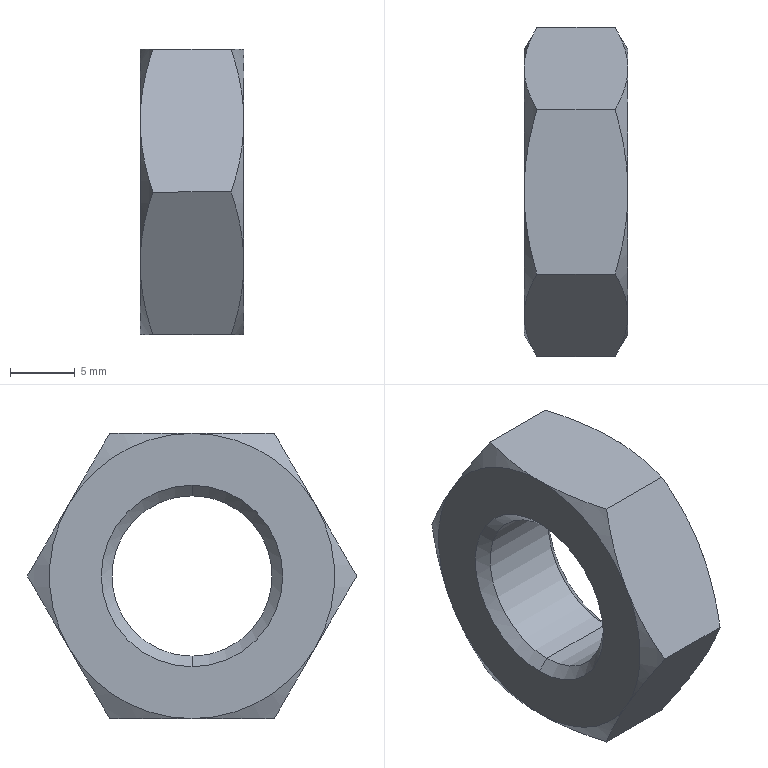Part | SolidWorks | features BaseBody 1 | 1 solid | 26 faces | box 8 x 25.403 x 22 mm | volume 2341 mm3 | cone 16 | plane 8 | cylinder 2 | commonest cylinder face diameters 12.376 x2
STEP:
#1=CARTESIAN_POINT('',(-3.188,0.,6.188));
#2=VERTEX_POINT('',#1);
#3=CARTESIAN_POINT('',(-3.188,0.,-6.188));
#4=VERTEX_POINT('',#3);
#5=CARTESIAN_POINT('',(-3.188,0.,0.));
#6=DIRECTION('',(1.,0.,0.));
#7=DIRECTION('',(0.,0.,-1.));
#8=AXIS2_PLACEMENT_3D('',#5,#6,#7);
#9=CIRCLE('',#8,6.188);
#10=EDGE_CURVE('',#2,#4,#9,.T.);
#11=ORIENTED_EDGE('',*,*,#10,.F.);
#12=CARTESIAN_POINT('',(3.188,0.,6.188));
#13=VERTEX_POINT('',#12);
#14=CARTESIAN_POINT('',(4.,0.,6.188));
#15=DIRECTION('',(1.,0.,0.));
#16=VECTOR('',#15,1000.);
#17=LINE('',#14,#16);
#18=EDGE_CURVE('',#2,#13,#17,.T.);
#19=ORIENTED_EDGE('',*,*,#18,.T.);
#20=CARTESIAN_POINT('',(3.188,0.,-6.188));
#21=VERTEX_POINT('',#20);
#22=CARTESIAN_POINT('',(3.188,0.,0.));
#23=DIRECTION('',(-1.,0.,0.));
#24=DIRECTION('',(0.,0.,-1.));
#25=AXIS2_PLACEMENT_3D('',#22,#23,#24);
#26=CIRCLE('',#25,6.188);
#27=EDGE_CURVE('',#21,#13,#26,.T.);
#28=ORIENTED_EDGE('',*,*,#27,.F.);
#29=CARTESIAN_POINT('',(4.,0.,-6.188));
#30=DIRECTION('',(1.,0.,0.));
#31=VECTOR('',#30,1000.);
#32=LINE('',#29,#31);
#33=EDGE_CURVE('',#4,#21,#32,.T.);
#34=ORIENTED_EDGE('',*,*,#33,.F.);
#35=EDGE_LOOP('',(#11,#19,#28,#34));
#36=FACE_OUTER_BOUND('',#35,.T.);
#37=CARTESIAN_POINT('',(4.,0.,0.));
#38=DIRECTION('',(1.,0.,0.));
#39=DIRECTION('',(0.,0.,-1.));
#40=AXIS2_PLACEMENT_3D('',#37,#38,#39);
#41=CYLINDRICAL_SURFACE('',#40,6.188);
#42=ADVANCED_FACE('',(#36),#41,.F.);
#43=ORIENTED_EDGE('',*,*,#10,.T.);
#44=CARTESIAN_POINT('',(-4.,0.,-7.));
#45=VERTEX_POINT('',#44);
#46=CARTESIAN_POINT('',(-4.,0.,-7.));
#47=DIRECTION('',(-0.7071,0.,-0.7071));
#48=VECTOR('',#47,1000.);
#49=LINE('',#46,#48);
#50=EDGE_CURVE('',#4,#45,#49,.T.);
#51=ORIENTED_EDGE('',*,*,#50,.T.);
#52=CARTESIAN_POINT('',(-4.,0.,7.));
#53=VERTEX_POINT('',#52);
#54=CARTESIAN_POINT('',(-4.,0.,0.));
#55=DIRECTION('',(1.,0.,0.));
#56=DIRECTION('',(0.,0.,1.));
#57=AXIS2_PLACEMENT_3D('',#54,#55,#56);
#58=CIRCLE('',#57,7.);
#59=EDGE_CURVE('',#53,#45,#58,.T.);
#60=ORIENTED_EDGE('',*,*,#59,.F.);
#61=CARTESIAN_POINT('',(-4.,0.,7.));
#62=DIRECTION('',(-0.7071,0.,0.7071));
#63=VECTOR('',#62,1000.);
#64=LINE('',#61,#63);
#65=EDGE_CURVE('',#2,#53,#64,.T.);
#66=ORIENTED_EDGE('',*,*,#65,.F.);
#67=EDGE_LOOP('',(#43,#51,#60,#66));
#68=FACE_OUTER_BOUND('',#67,.T.);
#69=CARTESIAN_POINT('',(-4.,0.,0.));
#70=DIRECTION('',(-1.,0.,0.));
#71=DIRECTION('',(0.,0.,1.));
#72=AXIS2_PLACEMENT_3D('',#69,#70,#71);
#73=CONICAL_SURFACE('',#72,7.,0.7854);
#74=ADVANCED_FACE('',(#68),#73,.F.);
#75=ORIENTED_EDGE('',*,*,#27,.T.);
#76=CARTESIAN_POINT('',(4.,0.,7.));
#77=VERTEX_POINT('',#76);
#78=CARTESIAN_POINT('',(4.,0.,7.));
#79=DIRECTION('',(0.7071,0.,0.7071));
#80=VECTOR('',#79,1000.);
#81=LINE('',#78,#80);
#82=EDGE_CURVE('',#13,#77,#81,.T.);
#83=ORIENTED_EDGE('',*,*,#82,.T.);
#84=CARTESIAN_POINT('',(4.,0.,-7.));
#85=VERTEX_POINT('',#84);
#86=CARTESIAN_POINT('',(4.,0.,0.));
#87=DIRECTION('',(-1.,0.,0.));
#88=DIRECTION('',(0.,0.,-1.));
#89=AXIS2_PLACEMENT_3D('',#86,#87,#88);
#90=CIRCLE('',#89,7.);
#91=EDGE_CURVE('',#85,#77,#90,.T.);
#92=ORIENTED_EDGE('',*,*,#91,.F.);
#93=CARTESIAN_POINT('',(4.,0.,-7.));
#94=DIRECTION('',(0.7071,0.,-0.7071));
#95=VECTOR('',#94,1000.);
#96=LINE('',#93,#95);
#97=EDGE_CURVE('',#21,#85,#96,.T.);
#98=ORIENTED_EDGE('',*,*,#97,.F.);
#99=EDGE_LOOP('',(#75,#83,#92,#98));
#100=FACE_OUTER_BOUND('',#99,.T.);
#101=CARTESIAN_POINT('',(4.,0.,0.));
#102=DIRECTION('',(1.,0.,0.));
#103=DIRECTION('',(0.,0.,-1.));
#104=AXIS2_PLACEMENT_3D('',#101,#102,#103);
#105=CONICAL_SURFACE('',#104,7.,0.7854);
#106=ADVANCED_FACE('',(#100),#105,.F.);
#107=ORIENTED_EDGE('',*,*,#18,.F.);
#108=CARTESIAN_POINT('',(-3.188,0.,0.));
#109=DIRECTION('',(1.,0.,0.));
#110=DIRECTION('',(0.,0.,-1.));
#111=AXIS2_PLACEMENT_3D('',#108,#109,#110);
#112=CIRCLE('',#111,6.188);
#113=EDGE_CURVE('',#4,#2,#112,.T.);
#114=ORIENTED_EDGE('',*,*,#113,.F.);
#115=ORIENTED_EDGE('',*,*,#33,.T.);
#116=CARTESIAN_POINT('',(3.188,0.,0.));
#117=DIRECTION('',(-1.,0.,0.));
#118=DIRECTION('',(0.,0.,-1.));
#119=AXIS2_PLACEMENT_3D('',#116,#117,#118);
#120=CIRCLE('',#119,6.188);
#121=EDGE_CURVE('',#13,#21,#120,.T.);
#122=ORIENTED_EDGE('',*,*,#121,.F.);
#123=EDGE_LOOP('',(#107,#114,#115,#122));
#124=FACE_OUTER_BOUND('',#123,.T.);
#125=CARTESIAN_POINT('',(4.,0.,0.));
#126=DIRECTION('',(1.,0.,0.));
#127=DIRECTION('',(0.,0.,-1.));
#128=AXIS2_PLACEMENT_3D('',#125,#126,#127);
#129=CYLINDRICAL_SURFACE('',#128,6.188);
#130=ADVANCED_FACE('',(#124),#129,.F.);
#131=ORIENTED_EDGE('',*,*,#50,.F.);
#132=ORIENTED_EDGE('',*,*,#113,.T.);
#133=ORIENTED_EDGE('',*,*,#65,.T.);
#134=CARTESIAN_POINT('',(-4.,0.,0.));
#135=DIRECTION('',(1.,0.,0.));
#136=DIRECTION('',(0.,0.,1.));
#137=AXIS2_PLACEMENT_3D('',#134,#135,#136);
#138=CIRCLE('',#137,7.);
#139=EDGE_CURVE('',#45,#53,#138,.T.);
#140=ORIENTED_EDGE('',*,*,#139,.F.);
#141=EDGE_LOOP('',(#131,#132,#133,#140));
#142=FACE_OUTER_BOUND('',#141,.T.);
#143=CARTESIAN_POINT('',(-4.,0.,0.));
#144=DIRECTION('',(-1.,0.,0.));
#145=DIRECTION('',(0.,0.,1.));
#146=AXIS2_PLACEMENT_3D('',#143,#144,#145);
#147=CONICAL_SURFACE('',#146,7.,0.7854);
#148=ADVANCED_FACE('',(#142),#147,.F.);
#149=ORIENTED_EDGE('',*,*,#82,.F.);
#150=ORIENTED_EDGE('',*,*,#121,.T.);
#151=ORIENTED_EDGE('',*,*,#97,.T.);
#152=CARTESIAN_POINT('',(4.,0.,0.));
#153=DIRECTION('',(-1.,0.,0.));
#154=DIRECTION('',(0.,0.,-1.));
#155=AXIS2_PLACEMENT_3D('',#152,#153,#154);
#156=CIRCLE('',#155,7.);
#157=EDGE_CURVE('',#77,#85,#156,.T.);
#158=ORIENTED_EDGE('',*,*,#157,.F.);
#159=EDGE_LOOP('',(#149,#150,#151,#158));
#160=FACE_OUTER_BOUND('',#159,.T.);
#161=CARTESIAN_POINT('',(4.,0.,0.));
#162=DIRECTION('',(1.,0.,0.));
#163=DIRECTION('',(0.,0.,-1.));
#164=AXIS2_PLACEMENT_3D('',#161,#162,#163);
#165=CONICAL_SURFACE('',#164,7.,0.7854);
#166=ADVANCED_FACE('',(#160),#165,.F.);
#167=CARTESIAN_POINT('',(-4.,-9.526,-5.5));
#168=VERTEX_POINT('',#167);
#169=CARTESIAN_POINT('',(-4.,0.,-11.));
#170=VERTEX_POINT('',#169);
#171=CARTESIAN_POINT('',(-4.,0.,0.));
#172=DIRECTION('',(1.,0.,0.));
#173=DIRECTION('',(0.,0.,-1.));
#174=AXIS2_PLACEMENT_3D('',#171,#172,#173);
#175=CIRCLE('',#174,11.);
#176=EDGE_CURVE('',#168,#170,#175,.T.);
#177=ORIENTED_EDGE('',*,*,#176,.F.);
#178=CARTESIAN_POINT('',(-4.,-9.526,5.5));
#179=VERTEX_POINT('',#178);
#180=CARTESIAN_POINT('',(-4.,0.,0.));
#181=DIRECTION('',(1.,0.,0.));
#182=DIRECTION('',(0.,0.,-1.));
#183=AXIS2_PLACEMENT_3D('',#180,#181,#182);
#184=CIRCLE('',#183,11.);
#185=EDGE_CURVE('',#179,#168,#184,.T.);
#186=ORIENTED_EDGE('',*,*,#185,.F.);
#187=CARTESIAN_POINT('',(-4.,0.,11.));
#188=VERTEX_POINT('',#187);
#189=CARTESIAN_POINT('',(-4.,0.,0.));
#190=DIRECTION('',(1.,0.,0.));
#191=DIRECTION('',(0.,0.,-1.));
#192=AXIS2_PLACEMENT_3D('',#189,#190,#191);
#193=CIRCLE('',#192,11.);
#194=EDGE_CURVE('',#188,#179,#193,.T.);
#195=ORIENTED_EDGE('',*,*,#194,.F.);
#196=CARTESIAN_POINT('',(-4.,9.526,5.5));
#197=VERTEX_POINT('',#196);
#198=CARTESIAN_POINT('',(-4.,0.,0.));
#199=DIRECTION('',(1.,0.,0.));
#200=DIRECTION('',(0.,0.,-1.));
#201=AXIS2_PLACEMENT_3D('',#198,#199,#200);
#202=CIRCLE('',#201,11.);
#203=EDGE_CURVE('',#197,#188,#202,.T.);
#204=ORIENTED_EDGE('',*,*,#203,.F.);
#205=CARTESIAN_POINT('',(-4.,9.526,-5.5));
#206=VERTEX_POINT('',#205);
#207=CARTESIAN_POINT('',(-4.,0.,0.));
#208=DIRECTION('',(1.,0.,0.));
#209=DIRECTION('',(0.,0.,-1.));
#210=AXIS2_PLACEMENT_3D('',#207,#208,#209);
#211=CIRCLE('',#210,11.);
#212=EDGE_CURVE('',#206,#197,#211,.T.);
#213=ORIENTED_EDGE('',*,*,#212,.F.);
#214=CARTESIAN_POINT('',(-4.,0.,0.));
#215=DIRECTION('',(1.,0.,0.));
#216=DIRECTION('',(0.,0.,-1.));
#217=AXIS2_PLACEMENT_3D('',#214,#215,#216);
#218=CIRCLE('',#217,11.);
#219=EDGE_CURVE('',#170,#206,#218,.T.);
#220=ORIENTED_EDGE('',*,*,#219,.F.);
#221=EDGE_LOOP('',(#177,#186,#195,#204,#213,#220));
#222=FACE_OUTER_BOUND('',#221,.T.);
#223=ORIENTED_EDGE('',*,*,#59,.T.);
#224=ORIENTED_EDGE('',*,*,#139,.T.);
#225=EDGE_LOOP('',(#223,#224));
#226=FACE_BOUND('',#225,.T.);
#227=CARTESIAN_POINT('',(-4.,0.,0.));
#228=DIRECTION('',(1.,0.,0.));
#229=DIRECTION('',(0.,0.,-1.));
#230=AXIS2_PLACEMENT_3D('',#227,#228,#229);
#231=PLANE('',#230);
#232=ADVANCED_FACE('',(#222,#226),#231,.F.);
#233=CARTESIAN_POINT('',(4.,0.,11.));
#234=VERTEX_POINT('',#233);
#235=CARTESIAN_POINT('',(4.,-9.526,5.5));
#236=VERTEX_POINT('',#235);
#237=CARTESIAN_POINT('',(4.,0.,0.));
#238=DIRECTION('',(1.,0.,0.));
#239=DIRECTION('',(0.,0.,1.));
#240=AXIS2_PLACEMENT_3D('',#237,#238,#239);
#241=CIRCLE('',#240,11.);
#242=EDGE_CURVE('',#234,#236,#241,.T.);
#243=ORIENTED_EDGE('',*,*,#242,.T.);
#244=CARTESIAN_POINT('',(4.,-9.526,-5.5));
#245=VERTEX_POINT('',#244);
#246=CARTESIAN_POINT('',(4.,0.,0.));
#247=DIRECTION('',(1.,0.,0.));
#248=DIRECTION('',(0.,0.,1.));
#249=AXIS2_PLACEMENT_3D('',#246,#247,#248);
#250=CIRCLE('',#249,11.);
#251=EDGE_CURVE('',#236,#245,#250,.T.);
#252=ORIENTED_EDGE('',*,*,#251,.T.);
#253=CARTESIAN_POINT('',(4.,0.,-11.));
#254=VERTEX_POINT('',#253);
#255=CARTESIAN_POINT('',(4.,0.,0.));
#256=DIRECTION('',(1.,0.,0.));
#257=DIRECTION('',(0.,0.,1.));
#258=AXIS2_PLACEMENT_3D('',#255,#256,#257);
#259=CIRCLE('',#258,11.);
#260=EDGE_CURVE('',#245,#254,#259,.T.);
#261=ORIENTED_EDGE('',*,*,#260,.T.);
#262=CARTESIAN_POINT('',(4.,9.526,-5.5));
#263=VERTEX_POINT('',#262);
#264=CARTESIAN_POINT('',(4.,0.,0.));
#265=DIRECTION('',(1.,0.,0.));
#266=DIRECTION('',(0.,0.,1.));
#267=AXIS2_PLACEMENT_3D('',#264,#265,#266);
#268=CIRCLE('',#267,11.);
#269=EDGE_CURVE('',#254,#263,#268,.T.);
#270=ORIENTED_EDGE('',*,*,#269,.T.);
#271=CARTESIAN_POINT('',(4.,9.526,5.5));
#272=VERTEX_POINT('',#271);
#273=CARTESIAN_POINT('',(4.,0.,0.));
#274=DIRECTION('',(1.,0.,0.));
#275=DIRECTION('',(0.,0.,1.));
#276=AXIS2_PLACEMENT_3D('',#273,#274,#275);
#277=CIRCLE('',#276,11.);
#278=EDGE_CURVE('',#263,#272,#277,.T.);
#279=ORIENTED_EDGE('',*,*,#278,.T.);
#280=CARTESIAN_POINT('',(4.,0.,0.));
#281=DIRECTION('',(1.,0.,0.));
#282=DIRECTION('',(0.,0.,1.));
#283=AXIS2_PLACEMENT_3D('',#280,#281,#282);
#284=CIRCLE('',#283,11.);
#285=EDGE_CURVE('',#272,#234,#284,.T.);
#286=ORIENTED_EDGE('',*,*,#285,.T.);
#287=EDGE_LOOP('',(#243,#252,#261,#270,#279,#286));
#288=FACE_OUTER_BOUND('',#287,.T.);
#289=ORIENTED_EDGE('',*,*,#91,.T.);
#290=ORIENTED_EDGE('',*,*,#157,.T.);
#291=EDGE_LOOP('',(#289,#290));
#292=FACE_BOUND('',#291,.T.);
#293=CARTESIAN_POINT('',(4.,0.,0.));
#294=DIRECTION('',(1.,0.,0.));
#295=DIRECTION('',(0.,0.,-1.));
#296=AXIS2_PLACEMENT_3D('',#293,#294,#295);
#297=PLANE('',#296);
#298=ADVANCED_FACE('',(#288,#292),#297,.T.);
#299=CARTESIAN_POINT('',(-3.018,6.351,-11.));
#300=VERTEX_POINT('',#299);
#301=CARTESIAN_POINT('',(-4.,9.526,-5.5));
#302=CARTESIAN_POINT('',(-4.,8.984,-6.439));
#303=CARTESIAN_POINT('',(-3.906,8.45,-7.365));
#304=CARTESIAN_POINT('',(-3.564,7.392,-9.196));
#305=CARTESIAN_POINT('',(-3.317,6.87,-10.102));
#306=CARTESIAN_POINT('',(-3.018,6.351,-11.));
#307=B_SPLINE_CURVE_WITH_KNOTS('',3,(#301,#302,#303,#304,#305,#306),.UNSPECIFIED.,.F.,.F.,(4,2,4),(0.,0.003213,0.006426),.UNSPECIFIED.);
#308=EDGE_CURVE('',#206,#300,#307,.T.);
#309=ORIENTED_EDGE('',*,*,#308,.T.);
#310=CARTESIAN_POINT('',(-3.018,6.351,-11.));
#311=CARTESIAN_POINT('',(-3.317,5.313,-11.));
#312=CARTESIAN_POINT('',(-3.564,4.268,-11.));
#313=CARTESIAN_POINT('',(-3.906,2.153,-11.));
#314=CARTESIAN_POINT('',(-4.,1.084,-11.));
#315=CARTESIAN_POINT('',(-4.,0.,-11.));
#316=B_SPLINE_CURVE_WITH_KNOTS('',3,(#310,#311,#312,#313,#314,#315),.UNSPECIFIED.,.F.,.F.,(4,2,4),(0.,0.003213,0.006426),.UNSPECIFIED.);
#317=EDGE_CURVE('',#300,#170,#316,.T.);
#318=ORIENTED_EDGE('',*,*,#317,.T.);
#319=ORIENTED_EDGE('',*,*,#219,.T.);
#320=EDGE_LOOP('',(#309,#318,#319));
#321=FACE_OUTER_BOUND('',#320,.T.);
#322=CARTESIAN_POINT('',(-3.012,0.,0.));
#323=DIRECTION('',(1.,0.,0.));
#324=DIRECTION('',(0.,0.,-1.));
#325=AXIS2_PLACEMENT_3D('',#322,#323,#324);
#326=CONICAL_SURFACE('',#325,12.712,1.047);
#327=ADVANCED_FACE('',(#321),#326,.T.);
#328=CARTESIAN_POINT('',(-3.018,-6.351,-11.));
#329=VERTEX_POINT('',#328);
#330=CARTESIAN_POINT('',(-4.,0.,-11.));
#331=CARTESIAN_POINT('',(-4.,-1.084,-11.));
#332=CARTESIAN_POINT('',(-3.906,-2.153,-11.));
#333=CARTESIAN_POINT('',(-3.564,-4.268,-11.));
#334=CARTESIAN_POINT('',(-3.317,-5.313,-11.));
#335=CARTESIAN_POINT('',(-3.018,-6.351,-11.));
#336=B_SPLINE_CURVE_WITH_KNOTS('',3,(#330,#331,#332,#333,#334,#335),.UNSPECIFIED.,.F.,.F.,(4,2,4),(0.,0.003213,0.006426),.UNSPECIFIED.);
#337=EDGE_CURVE('',#170,#329,#336,.T.);
#338=ORIENTED_EDGE('',*,*,#337,.T.);
#339=CARTESIAN_POINT('',(-3.018,-6.351,-11.));
#340=CARTESIAN_POINT('',(-3.317,-6.87,-10.102));
#341=CARTESIAN_POINT('',(-3.564,-7.392,-9.196));
#342=CARTESIAN_POINT('',(-3.906,-8.45,-7.365));
#343=CARTESIAN_POINT('',(-4.,-8.984,-6.439));
#344=CARTESIAN_POINT('',(-4.,-9.526,-5.5));
#345=B_SPLINE_CURVE_WITH_KNOTS('',3,(#339,#340,#341,#342,#343,#344),.UNSPECIFIED.,.F.,.F.,(4,2,4),(0.,0.003213,0.006426),.UNSPECIFIED.);
#346=EDGE_CURVE('',#329,#168,#345,.T.);
#347=ORIENTED_EDGE('',*,*,#346,.T.);
#348=ORIENTED_EDGE('',*,*,#176,.T.);
#349=EDGE_LOOP('',(#338,#347,#348));
#350=FACE_OUTER_BOUND('',#349,.T.);
#351=CARTESIAN_POINT('',(-3.012,0.,0.));
#352=DIRECTION('',(1.,0.,0.));
#353=DIRECTION('',(0.,0.,-1.));
#354=AXIS2_PLACEMENT_3D('',#351,#352,#353);
#355=CONICAL_SURFACE('',#354,12.712,1.047);
#356=ADVANCED_FACE('',(#350),#355,.T.);
#357=CARTESIAN_POINT('',(-3.018,-12.702,-0.000000043));
#358=VERTEX_POINT('',#357);
#359=CARTESIAN_POINT('',(-4.,-9.526,-5.5));
#360=CARTESIAN_POINT('',(-4.,-10.068,-4.561));
#361=CARTESIAN_POINT('',(-3.906,-10.603,-3.635));
#362=CARTESIAN_POINT('',(-3.564,-11.66,-1.804));
#363=CARTESIAN_POINT('',(-3.317,-12.183,-0.8985));
#364=CARTESIAN_POINT('',(-3.018,-12.702,-0.000000043));
#365=B_SPLINE_CURVE_WITH_KNOTS('',3,(#359,#360,#361,#362,#363,#364),.UNSPECIFIED.,.F.,.F.,(4,2,4),(0.,0.003213,0.006426),.UNSPECIFIED.);
#366=EDGE_CURVE('',#168,#358,#365,.T.);
#367=ORIENTED_EDGE('',*,*,#366,.T.);
#368=CARTESIAN_POINT('',(-3.018,-12.702,-0.000000043));
#369=CARTESIAN_POINT('',(-3.317,-12.183,0.8985));
#370=CARTESIAN_POINT('',(-3.564,-11.66,1.804));
#371=CARTESIAN_POINT('',(-3.906,-10.603,3.635));
#372=CARTESIAN_POINT('',(-4.,-10.068,4.561));
#373=CARTESIAN_POINT('',(-4.,-9.526,5.5));
#374=B_SPLINE_CURVE_WITH_KNOTS('',3,(#368,#369,#370,#371,#372,#373),.UNSPECIFIED.,.F.,.F.,(4,2,4),(0.,0.003213,0.006426),.UNSPECIFIED.);
#375=EDGE_CURVE('',#358,#179,#374,.T.);
#376=ORIENTED_EDGE('',*,*,#375,.T.);
#377=ORIENTED_EDGE('',*,*,#185,.T.);
#378=EDGE_LOOP('',(#367,#376,#377));
#379=FACE_OUTER_BOUND('',#378,.T.);
#380=CARTESIAN_POINT('',(-3.012,0.,0.));
#381=DIRECTION('',(1.,0.,0.));
#382=DIRECTION('',(0.,0.,-1.));
#383=AXIS2_PLACEMENT_3D('',#380,#381,#382);
#384=CONICAL_SURFACE('',#383,12.712,1.047);
#385=ADVANCED_FACE('',(#379),#384,.T.);
#386=CARTESIAN_POINT('',(-3.018,-6.351,11.));
#387=VERTEX_POINT('',#386);
#388=CARTESIAN_POINT('',(-4.,-9.526,5.5));
#389=CARTESIAN_POINT('',(-4.,-8.984,6.439));
#390=CARTESIAN_POINT('',(-3.906,-8.45,7.365));
#391=CARTESIAN_POINT('',(-3.564,-7.392,9.196));
#392=CARTESIAN_POINT('',(-3.317,-6.87,10.102));
#393=CARTESIAN_POINT('',(-3.018,-6.351,11.));
#394=B_SPLINE_CURVE_WITH_KNOTS('',3,(#388,#389,#390,#391,#392,#393),.UNSPECIFIED.,.F.,.F.,(4,2,4),(0.,0.003213,0.006426),.UNSPECIFIED.);
#395=EDGE_CURVE('',#179,#387,#394,.T.);
#396=ORIENTED_EDGE('',*,*,#395,.T.);
#397=CARTESIAN_POINT('',(-3.018,-6.351,11.));
#398=CARTESIAN_POINT('',(-3.317,-5.313,11.));
#399=CARTESIAN_POINT('',(-3.564,-4.268,11.));
#400=CARTESIAN_POINT('',(-3.906,-2.153,11.));
#401=CARTESIAN_POINT('',(-4.,-1.084,11.));
#402=CARTESIAN_POINT('',(-4.,0.,11.));
#403=B_SPLINE_CURVE_WITH_KNOTS('',3,(#397,#398,#399,#400,#401,#402),.UNSPECIFIED.,.F.,.F.,(4,2,4),(0.,0.003213,0.006426),.UNSPECIFIED.);
#404=EDGE_CURVE('',#387,#188,#403,.T.);
#405=ORIENTED_EDGE('',*,*,#404,.T.);
#406=ORIENTED_EDGE('',*,*,#194,.T.);
#407=EDGE_LOOP('',(#396,#405,#406));
#408=FACE_OUTER_BOUND('',#407,.T.);
#409=CARTESIAN_POINT('',(-3.012,0.,0.));
#410=DIRECTION('',(1.,0.,0.));
#411=DIRECTION('',(0.,0.,-1.));
#412=AXIS2_PLACEMENT_3D('',#409,#410,#411);
#413=CONICAL_SURFACE('',#412,12.712,1.047);
#414=ADVANCED_FACE('',(#408),#413,.T.);
#415=ORIENTED_EDGE('',*,*,#203,.T.);
#416=CARTESIAN_POINT('',(-3.018,6.351,11.));
#417=VERTEX_POINT('',#416);
#418=CARTESIAN_POINT('',(-4.,0.,11.));
#419=CARTESIAN_POINT('',(-4.,1.084,11.));
#420=CARTESIAN_POINT('',(-3.906,2.153,11.));
#421=CARTESIAN_POINT('',(-3.564,4.268,11.));
#422=CARTESIAN_POINT('',(-3.317,5.313,11.));
#423=CARTESIAN_POINT('',(-3.018,6.351,11.));
#424=B_SPLINE_CURVE_WITH_KNOTS('',3,(#418,#419,#420,#421,#422,#423),.UNSPECIFIED.,.F.,.F.,(4,2,4),(0.,0.003213,0.006426),.UNSPECIFIED.);
#425=EDGE_CURVE('',#188,#417,#424,.T.);
#426=ORIENTED_EDGE('',*,*,#425,.T.);
#427=CARTESIAN_POINT('',(-3.018,6.351,11.));
#428=CARTESIAN_POINT('',(-3.317,6.87,10.102));
#429=CARTESIAN_POINT('',(-3.564,7.392,9.196));
#430=CARTESIAN_POINT('',(-3.906,8.45,7.365));
#431=CARTESIAN_POINT('',(-4.,8.984,6.439));
#432=CARTESIAN_POINT('',(-4.,9.526,5.5));
#433=B_SPLINE_CURVE_WITH_KNOTS('',3,(#427,#428,#429,#430,#431,#432),.UNSPECIFIED.,.F.,.F.,(4,2,4),(0.,0.003213,0.006426),.UNSPECIFIED.);
#434=EDGE_CURVE('',#417,#197,#433,.T.);
#435=ORIENTED_EDGE('',*,*,#434,.T.);
#436=EDGE_LOOP('',(#415,#426,#435));
#437=FACE_OUTER_BOUND('',#436,.T.);
#438=CARTESIAN_POINT('',(-3.012,0.,0.));
#439=DIRECTION('',(1.,0.,0.));
#440=DIRECTION('',(0.,0.,-1.));
#441=AXIS2_PLACEMENT_3D('',#438,#439,#440);
#442=CONICAL_SURFACE('',#441,12.712,1.047);
#443=ADVANCED_FACE('',(#437),#442,.T.);
#444=CARTESIAN_POINT('',(-3.018,12.702,0.000000043));
#445=VERTEX_POINT('',#444);
#446=CARTESIAN_POINT('',(-4.,9.526,5.5));
#447=CARTESIAN_POINT('',(-4.,10.068,4.561));
#448=CARTESIAN_POINT('',(-3.906,10.603,3.635));
#449=CARTESIAN_POINT('',(-3.564,11.66,1.804));
#450=CARTESIAN_POINT('',(-3.317,12.183,0.8985));
#451=CARTESIAN_POINT('',(-3.018,12.702,0.000000043));
#452=B_SPLINE_CURVE_WITH_KNOTS('',3,(#446,#447,#448,#449,#450,#451),.UNSPECIFIED.,.F.,.F.,(4,2,4),(0.,0.003213,0.006426),.UNSPECIFIED.);
#453=EDGE_CURVE('',#197,#445,#452,.T.);
#454=ORIENTED_EDGE('',*,*,#453,.T.);
#455=CARTESIAN_POINT('',(-3.018,12.702,0.000000043));
#456=CARTESIAN_POINT('',(-3.317,12.183,-0.8985));
#457=CARTESIAN_POINT('',(-3.564,11.66,-1.804));
#458=CARTESIAN_POINT('',(-3.906,10.603,-3.635));
#459=CARTESIAN_POINT('',(-4.,10.068,-4.561));
#460=CARTESIAN_POINT('',(-4.,9.526,-5.5));
#461=B_SPLINE_CURVE_WITH_KNOTS('',3,(#455,#456,#457,#458,#459,#460),.UNSPECIFIED.,.F.,.F.,(4,2,4),(0.,0.003213,0.006426),.UNSPECIFIED.);
#462=EDGE_CURVE('',#445,#206,#461,.T.);
#463=ORIENTED_EDGE('',*,*,#462,.T.);
#464=ORIENTED_EDGE('',*,*,#212,.T.);
#465=EDGE_LOOP('',(#454,#463,#464));
#466=FACE_OUTER_BOUND('',#465,.T.);
#467=CARTESIAN_POINT('',(-3.012,0.,0.));
#468=DIRECTION('',(1.,0.,0.));
#469=DIRECTION('',(0.,0.,-1.));
#470=AXIS2_PLACEMENT_3D('',#467,#468,#469);
#471=CONICAL_SURFACE('',#470,12.712,1.047);
#472=ADVANCED_FACE('',(#466),#471,.T.);
#473=CARTESIAN_POINT('',(3.018,-12.702,0.000000043));
#474=VERTEX_POINT('',#473);
#475=CARTESIAN_POINT('',(4.,-9.526,5.5));
#476=CARTESIAN_POINT('',(4.,-10.068,4.561));
#477=CARTESIAN_POINT('',(3.906,-10.603,3.635));
#478=CARTESIAN_POINT('',(3.564,-11.66,1.804));
#479=CARTESIAN_POINT('',(3.317,-12.183,0.8985));
#480=CARTESIAN_POINT('',(3.018,-12.702,0.000000043));
#481=B_SPLINE_CURVE_WITH_KNOTS('',3,(#475,#476,#477,#478,#479,#480),.UNSPECIFIED.,.F.,.F.,(4,2,4),(0.,0.003213,0.006426),.UNSPECIFIED.);
#482=EDGE_CURVE('',#236,#474,#481,.T.);
#483=ORIENTED_EDGE('',*,*,#482,.T.);
#484=CARTESIAN_POINT('',(3.018,-12.702,0.000000043));
#485=CARTESIAN_POINT('',(3.317,-12.183,-0.8985));
#486=CARTESIAN_POINT('',(3.564,-11.66,-1.804));
#487=CARTESIAN_POINT('',(3.906,-10.603,-3.635));
#488=CARTESIAN_POINT('',(4.,-10.068,-4.561));
#489=CARTESIAN_POINT('',(4.,-9.526,-5.5));
#490=B_SPLINE_CURVE_WITH_KNOTS('',3,(#484,#485,#486,#487,#488,#489),.UNSPECIFIED.,.F.,.F.,(4,2,4),(0.,0.003213,0.006426),.UNSPECIFIED.);
#491=EDGE_CURVE('',#474,#245,#490,.T.);
#492=ORIENTED_EDGE('',*,*,#491,.T.);
#493=ORIENTED_EDGE('',*,*,#251,.F.);
#494=EDGE_LOOP('',(#483,#492,#493));
#495=FACE_OUTER_BOUND('',#494,.T.);
#496=CARTESIAN_POINT('',(3.012,0.,0.));
#497=DIRECTION('',(-1.,0.,0.));
#498=DIRECTION('',(0.,0.,1.));
#499=AXIS2_PLACEMENT_3D('',#496,#497,#498);
#500=CONICAL_SURFACE('',#499,12.712,1.047);
#501=ADVANCED_FACE('',(#495),#500,.T.);
#502=CARTESIAN_POINT('',(3.018,-6.351,11.));
#503=VERTEX_POINT('',#502);
#504=CARTESIAN_POINT('',(4.,0.,11.));
#505=CARTESIAN_POINT('',(4.,-1.084,11.));
#506=CARTESIAN_POINT('',(3.906,-2.153,11.));
#507=CARTESIAN_POINT('',(3.564,-4.268,11.));
#508=CARTESIAN_POINT('',(3.317,-5.313,11.));
#509=CARTESIAN_POINT('',(3.018,-6.351,11.));
#510=B_SPLINE_CURVE_WITH_KNOTS('',3,(#504,#505,#506,#507,#508,#509),.UNSPECIFIED.,.F.,.F.,(4,2,4),(0.,0.003213,0.006426),.UNSPECIFIED.);
#511=EDGE_CURVE('',#234,#503,#510,.T.);
#512=ORIENTED_EDGE('',*,*,#511,.T.);
#513=CARTESIAN_POINT('',(3.018,-6.351,11.));
#514=CARTESIAN_POINT('',(3.317,-6.87,10.102));
#515=CARTESIAN_POINT('',(3.564,-7.392,9.196));
#516=CARTESIAN_POINT('',(3.906,-8.45,7.365));
#517=CARTESIAN_POINT('',(4.,-8.984,6.439));
#518=CARTESIAN_POINT('',(4.,-9.526,5.5));
#519=B_SPLINE_CURVE_WITH_KNOTS('',3,(#513,#514,#515,#516,#517,#518),.UNSPECIFIED.,.F.,.F.,(4,2,4),(0.,0.003213,0.006426),.UNSPECIFIED.);
#520=EDGE_CURVE('',#503,#236,#519,.T.);
#521=ORIENTED_EDGE('',*,*,#520,.T.);
#522=ORIENTED_EDGE('',*,*,#242,.F.);
#523=EDGE_LOOP('',(#512,#521,#522));
#524=FACE_OUTER_BOUND('',#523,.T.);
#525=CARTESIAN_POINT('',(3.012,0.,0.));
#526=DIRECTION('',(-1.,0.,0.));
#527=DIRECTION('',(0.,0.,1.));
#528=AXIS2_PLACEMENT_3D('',#525,#526,#527);
#529=CONICAL_SURFACE('',#528,12.712,1.047);
#530=ADVANCED_FACE('',(#524),#529,.T.);
#531=CARTESIAN_POINT('',(3.018,6.351,11.));
#532=VERTEX_POINT('',#531);
#533=CARTESIAN_POINT('',(4.,9.526,5.5));
#534=CARTESIAN_POINT('',(4.,8.984,6.439));
#535=CARTESIAN_POINT('',(3.906,8.45,7.365));
#536=CARTESIAN_POINT('',(3.564,7.392,9.196));
#537=CARTESIAN_POINT('',(3.317,6.87,10.102));
#538=CARTESIAN_POINT('',(3.018,6.351,11.));
#539=B_SPLINE_CURVE_WITH_KNOTS('',3,(#533,#534,#535,#536,#537,#538),.UNSPECIFIED.,.F.,.F.,(4,2,4),(0.,0.003213,0.006426),.UNSPECIFIED.);
#540=EDGE_CURVE('',#272,#532,#539,.T.);
#541=ORIENTED_EDGE('',*,*,#540,.T.);
#542=CARTESIAN_POINT('',(3.018,6.351,11.));
#543=CARTESIAN_POINT('',(3.317,5.313,11.));
#544=CARTESIAN_POINT('',(3.564,4.268,11.));
#545=CARTESIAN_POINT('',(3.906,2.153,11.));
#546=CARTESIAN_POINT('',(4.,1.084,11.));
#547=CARTESIAN_POINT('',(4.,0.,11.));
#548=B_SPLINE_CURVE_WITH_KNOTS('',3,(#542,#543,#544,#545,#546,#547),.UNSPECIFIED.,.F.,.F.,(4,2,4),(0.,0.003213,0.006426),.UNSPECIFIED.);
#549=EDGE_CURVE('',#532,#234,#548,.T.);
#550=ORIENTED_EDGE('',*,*,#549,.T.);
#551=ORIENTED_EDGE('',*,*,#285,.F.);
#552=EDGE_LOOP('',(#541,#550,#551));
#553=FACE_OUTER_BOUND('',#552,.T.);
#554=CARTESIAN_POINT('',(3.012,0.,0.));
#555=DIRECTION('',(-1.,0.,0.));
#556=DIRECTION('',(0.,0.,1.));
#557=AXIS2_PLACEMENT_3D('',#554,#555,#556);
#558=CONICAL_SURFACE('',#557,12.712,1.047);
#559=ADVANCED_FACE('',(#553),#558,.T.);
#560=ORIENTED_EDGE('',*,*,#278,.F.);
#561=CARTESIAN_POINT('',(3.018,12.702,0.000000029));
#562=VERTEX_POINT('',#561);
#563=CARTESIAN_POINT('',(4.,9.526,-5.5));
#564=CARTESIAN_POINT('',(4.,10.068,-4.561));
#565=CARTESIAN_POINT('',(3.906,10.603,-3.635));
#566=CARTESIAN_POINT('',(3.564,11.66,-1.804));
#567=CARTESIAN_POINT('',(3.317,12.183,-0.8985));
#568=CARTESIAN_POINT('',(3.018,12.702,0.000000029));
#569=B_SPLINE_CURVE_WITH_KNOTS('',3,(#563,#564,#565,#566,#567,#568),.UNSPECIFIED.,.F.,.F.,(4,2,4),(0.,0.003213,0.006426),.UNSPECIFIED.);
#570=EDGE_CURVE('',#263,#562,#569,.T.);
#571=ORIENTED_EDGE('',*,*,#570,.T.);
#572=CARTESIAN_POINT('',(3.018,12.702,0.000000029));
#573=CARTESIAN_POINT('',(3.317,12.183,0.8985));
#574=CARTESIAN_POINT('',(3.564,11.66,1.804));
#575=CARTESIAN_POINT('',(3.906,10.603,3.635));
#576=CARTESIAN_POINT('',(4.,10.068,4.561));
#577=CARTESIAN_POINT('',(4.,9.526,5.5));
#578=B_SPLINE_CURVE_WITH_KNOTS('',3,(#572,#573,#574,#575,#576,#577),.UNSPECIFIED.,.F.,.F.,(4,2,4),(0.,0.003213,0.006426),.UNSPECIFIED.);
#579=EDGE_CURVE('',#562,#272,#578,.T.);
#580=ORIENTED_EDGE('',*,*,#579,.T.);
#581=EDGE_LOOP('',(#560,#571,#580));
#582=FACE_OUTER_BOUND('',#581,.T.);
#583=CARTESIAN_POINT('',(3.012,0.,0.));
#584=DIRECTION('',(-1.,0.,0.));
#585=DIRECTION('',(0.,0.,1.));
#586=AXIS2_PLACEMENT_3D('',#583,#584,#585);
#587=CONICAL_SURFACE('',#586,12.712,1.047);
#588=ADVANCED_FACE('',(#582),#587,.T.);
#589=ORIENTED_EDGE('',*,*,#269,.F.);
#590=CARTESIAN_POINT('',(3.018,6.351,-11.));
#591=VERTEX_POINT('',#590);
#592=CARTESIAN_POINT('',(4.,0.,-11.));
#593=CARTESIAN_POINT('',(4.,1.084,-11.));
#594=CARTESIAN_POINT('',(3.906,2.153,-11.));
#595=CARTESIAN_POINT('',(3.564,4.268,-11.));
#596=CARTESIAN_POINT('',(3.317,5.313,-11.));
#597=CARTESIAN_POINT('',(3.018,6.351,-11.));
#598=B_SPLINE_CURVE_WITH_KNOTS('',3,(#592,#593,#594,#595,#596,#597),.UNSPECIFIED.,.F.,.F.,(4,2,4),(0.,0.003213,0.006426),.UNSPECIFIED.);
#599=EDGE_CURVE('',#254,#591,#598,.T.);
#600=ORIENTED_EDGE('',*,*,#599,.T.);
#601=CARTESIAN_POINT('',(3.018,6.351,-11.));
#602=CARTESIAN_POINT('',(3.317,6.87,-10.102));
#603=CARTESIAN_POINT('',(3.564,7.392,-9.196));
#604=CARTESIAN_POINT('',(3.906,8.45,-7.365));
#605=CARTESIAN_POINT('',(4.,8.984,-6.439));
#606=CARTESIAN_POINT('',(4.,9.526,-5.5));
#607=B_SPLINE_CURVE_WITH_KNOTS('',3,(#601,#602,#603,#604,#605,#606),.UNSPECIFIED.,.F.,.F.,(4,2,4),(0.,0.003213,0.006426),.UNSPECIFIED.);
#608=EDGE_CURVE('',#591,#263,#607,.T.);
#609=ORIENTED_EDGE('',*,*,#608,.T.);
#610=EDGE_LOOP('',(#589,#600,#609));
#611=FACE_OUTER_BOUND('',#610,.T.);
#612=CARTESIAN_POINT('',(3.012,0.,0.));
#613=DIRECTION('',(-1.,0.,0.));
#614=DIRECTION('',(0.,0.,1.));
#615=AXIS2_PLACEMENT_3D('',#612,#613,#614);
#616=CONICAL_SURFACE('',#615,12.712,1.047);
#617=ADVANCED_FACE('',(#611),#616,.T.);
#618=ORIENTED_EDGE('',*,*,#260,.F.);
#619=CARTESIAN_POINT('',(3.018,-6.351,-11.));
#620=VERTEX_POINT('',#619);
#621=CARTESIAN_POINT('',(4.,-9.526,-5.5));
#622=CARTESIAN_POINT('',(4.,-8.984,-6.439));
#623=CARTESIAN_POINT('',(3.906,-8.45,-7.365));
#624=CARTESIAN_POINT('',(3.564,-7.392,-9.196));
#625=CARTESIAN_POINT('',(3.317,-6.87,-10.102));
#626=CARTESIAN_POINT('',(3.018,-6.351,-11.));
#627=B_SPLINE_CURVE_WITH_KNOTS('',3,(#621,#622,#623,#624,#625,#626),.UNSPECIFIED.,.F.,.F.,(4,2,4),(0.,0.003213,0.006426),.UNSPECIFIED.);
#628=EDGE_CURVE('',#245,#620,#627,.T.);
#629=ORIENTED_EDGE('',*,*,#628,.T.);
#630=CARTESIAN_POINT('',(3.018,-6.351,-11.));
#631=CARTESIAN_POINT('',(3.317,-5.313,-11.));
#632=CARTESIAN_POINT('',(3.564,-4.268,-11.));
#633=CARTESIAN_POINT('',(3.906,-2.153,-11.));
#634=CARTESIAN_POINT('',(4.,-1.084,-11.));
#635=CARTESIAN_POINT('',(4.,0.,-11.));
#636=B_SPLINE_CURVE_WITH_KNOTS('',3,(#630,#631,#632,#633,#634,#635),.UNSPECIFIED.,.F.,.F.,(4,2,4),(0.,0.003213,0.006426),.UNSPECIFIED.);
#637=EDGE_CURVE('',#620,#254,#636,.T.);
#638=ORIENTED_EDGE('',*,*,#637,.T.);
#639=EDGE_LOOP('',(#618,#629,#638));
#640=FACE_OUTER_BOUND('',#639,.T.);
#641=CARTESIAN_POINT('',(3.012,0.,0.));
#642=DIRECTION('',(-1.,0.,0.));
#643=DIRECTION('',(0.,0.,1.));
#644=AXIS2_PLACEMENT_3D('',#641,#642,#643);
#645=CONICAL_SURFACE('',#644,12.712,1.047);
#646=ADVANCED_FACE('',(#640),#645,.T.);
#647=ORIENTED_EDGE('',*,*,#337,.F.);
#648=ORIENTED_EDGE('',*,*,#317,.F.);
#649=CARTESIAN_POINT('',(4.,6.351,-11.));
#650=DIRECTION('',(-1.,0.,0.));
#651=VECTOR('',#650,1000.);
#652=LINE('',#649,#651);
#653=EDGE_CURVE('',#591,#300,#652,.T.);
#654=ORIENTED_EDGE('',*,*,#653,.F.);
#655=ORIENTED_EDGE('',*,*,#599,.F.);
#656=ORIENTED_EDGE('',*,*,#637,.F.);
#657=CARTESIAN_POINT('',(4.,-6.351,-11.));
#658=DIRECTION('',(1.,0.,0.));
#659=VECTOR('',#658,1000.);
#660=LINE('',#657,#659);
#661=EDGE_CURVE('',#329,#620,#660,.T.);
#662=ORIENTED_EDGE('',*,*,#661,.F.);
#663=EDGE_LOOP('',(#647,#648,#654,#655,#656,#662));
#664=FACE_OUTER_BOUND('',#663,.T.);
#665=CARTESIAN_POINT('',(4.,-6.351,-11.));
#666=DIRECTION('',(0.,0.,1.));
#667=DIRECTION('',(1.,0.,0.));
#668=AXIS2_PLACEMENT_3D('',#665,#666,#667);
#669=PLANE('',#668);
#670=ADVANCED_FACE('',(#664),#669,.F.);
#671=ORIENTED_EDGE('',*,*,#308,.F.);
#672=ORIENTED_EDGE('',*,*,#462,.F.);
#673=CARTESIAN_POINT('',(4.,12.702,0.));
#674=DIRECTION('',(-1.,0.,0.));
#675=VECTOR('',#674,1000.);
#676=LINE('',#673,#675);
#677=EDGE_CURVE('',#562,#445,#676,.T.);
#678=ORIENTED_EDGE('',*,*,#677,.F.);
#679=ORIENTED_EDGE('',*,*,#570,.F.);
#680=ORIENTED_EDGE('',*,*,#608,.F.);
#681=ORIENTED_EDGE('',*,*,#653,.T.);
#682=EDGE_LOOP('',(#671,#672,#678,#679,#680,#681));
#683=FACE_OUTER_BOUND('',#682,.T.);
#684=CARTESIAN_POINT('',(4.,6.351,-11.));
#685=DIRECTION('',(0.,-0.866,0.5));
#686=DIRECTION('',(0.,-0.5,-0.866));
#687=AXIS2_PLACEMENT_3D('',#684,#685,#686);
#688=PLANE('',#687);
#689=ADVANCED_FACE('',(#683),#688,.F.);
#690=ORIENTED_EDGE('',*,*,#366,.F.);
#691=ORIENTED_EDGE('',*,*,#346,.F.);
#692=ORIENTED_EDGE('',*,*,#661,.T.);
#693=ORIENTED_EDGE('',*,*,#628,.F.);
#694=ORIENTED_EDGE('',*,*,#491,.F.);
#695=CARTESIAN_POINT('',(4.,-12.702,0.));
#696=DIRECTION('',(1.,0.,0.));
#697=VECTOR('',#696,1000.);
#698=LINE('',#695,#697);
#699=EDGE_CURVE('',#358,#474,#698,.T.);
#700=ORIENTED_EDGE('',*,*,#699,.F.);
#701=EDGE_LOOP('',(#690,#691,#692,#693,#694,#700));
#702=FACE_OUTER_BOUND('',#701,.T.);
#703=CARTESIAN_POINT('',(4.,-12.702,0.));
#704=DIRECTION('',(0.,0.866,0.5));
#705=DIRECTION('',(0.,-0.5,0.866));
#706=AXIS2_PLACEMENT_3D('',#703,#704,#705);
#707=PLANE('',#706);
#708=ADVANCED_FACE('',(#702),#707,.F.);
#709=ORIENTED_EDGE('',*,*,#395,.F.);
#710=ORIENTED_EDGE('',*,*,#375,.F.);
#711=ORIENTED_EDGE('',*,*,#699,.T.);
#712=ORIENTED_EDGE('',*,*,#482,.F.);
#713=ORIENTED_EDGE('',*,*,#520,.F.);
#714=CARTESIAN_POINT('',(4.,-6.351,11.));
#715=DIRECTION('',(1.,0.,0.));
#716=VECTOR('',#715,1000.);
#717=LINE('',#714,#716);
#718=EDGE_CURVE('',#387,#503,#717,.T.);
#719=ORIENTED_EDGE('',*,*,#718,.F.);
#720=EDGE_LOOP('',(#709,#710,#711,#712,#713,#719));
#721=FACE_OUTER_BOUND('',#720,.T.);
#722=CARTESIAN_POINT('',(4.,-6.351,11.));
#723=DIRECTION('',(0.,0.866,-0.5));
#724=DIRECTION('',(0.,0.5,0.866));
#725=AXIS2_PLACEMENT_3D('',#722,#723,#724);
#726=PLANE('',#725);
#727=ADVANCED_FACE('',(#721),#726,.F.);
#728=ORIENTED_EDGE('',*,*,#425,.F.);
#729=ORIENTED_EDGE('',*,*,#404,.F.);
#730=ORIENTED_EDGE('',*,*,#718,.T.);
#731=ORIENTED_EDGE('',*,*,#511,.F.);
#732=ORIENTED_EDGE('',*,*,#549,.F.);
#733=CARTESIAN_POINT('',(4.,6.351,11.));
#734=DIRECTION('',(1.,0.,0.));
#735=VECTOR('',#734,1000.);
#736=LINE('',#733,#735);
#737=EDGE_CURVE('',#417,#532,#736,.T.);
#738=ORIENTED_EDGE('',*,*,#737,.F.);
#739=EDGE_LOOP('',(#728,#729,#730,#731,#732,#738));
#740=FACE_OUTER_BOUND('',#739,.T.);
#741=CARTESIAN_POINT('',(4.,6.351,11.));
#742=DIRECTION('',(0.,0.,-1.));
#743=DIRECTION('',(-1.,0.,0.));
#744=AXIS2_PLACEMENT_3D('',#741,#742,#743);
#745=PLANE('',#744);
#746=ADVANCED_FACE('',(#740),#745,.F.);
#747=ORIENTED_EDGE('',*,*,#453,.F.);
#748=ORIENTED_EDGE('',*,*,#434,.F.);
#749=ORIENTED_EDGE('',*,*,#737,.T.);
#750=ORIENTED_EDGE('',*,*,#540,.F.);
#751=ORIENTED_EDGE('',*,*,#579,.F.);
#752=ORIENTED_EDGE('',*,*,#677,.T.);
#753=EDGE_LOOP('',(#747,#748,#749,#750,#751,#752));
#754=FACE_OUTER_BOUND('',#753,.T.);
#755=CARTESIAN_POINT('',(4.,12.702,0.));
#756=DIRECTION('',(0.,-0.866,-0.5));
#757=DIRECTION('',(0.,0.5,-0.866));
#758=AXIS2_PLACEMENT_3D('',#755,#756,#757);
#759=PLANE('',#758);
#760=ADVANCED_FACE('',(#754),#759,.F.);
#761=CLOSED_SHELL('',(#42,#74,#106,#130,#148,#166,#232,#298,#327,#356,#385,#414,#443,#472,#501,#530,#559,#588,#617,#646,#670,#689,#708,#727,#746,#760));
#762=MANIFOLD_SOLID_BREP('',#761);
#763=CARTESIAN_POINT('',(0.,0.,0.));
#764=DIRECTION('',(0.,0.,1.));
#765=DIRECTION('',(1.,0.,0.));
#766=AXIS2_PLACEMENT_3D('',#763,#764,#765);
#767=(LENGTH_UNIT()NAMED_UNIT(*)SI_UNIT(.MILLI.,.METRE.));
#768=UNCERTAINTY_MEASURE_WITH_UNIT(LENGTH_MEASURE(0.00001),#767,'','');
#769=(NAMED_UNIT(*)PLANE_ANGLE_UNIT()SI_UNIT($,.RADIAN.));
#770=(NAMED_UNIT(*)SI_UNIT($,.STERADIAN.)SOLID_ANGLE_UNIT());
#771=(GEOMETRIC_REPRESENTATION_CONTEXT(3)GLOBAL_UNCERTAINTY_ASSIGNED_CONTEXT((#768))GLOBAL_UNIT_ASSIGNED_CONTEXT((#767,#769,#770))REPRESENTATION_CONTEXT('',''));
#772=ADVANCED_BREP_SHAPE_REPRESENTATION('',(#762,#766),#771);